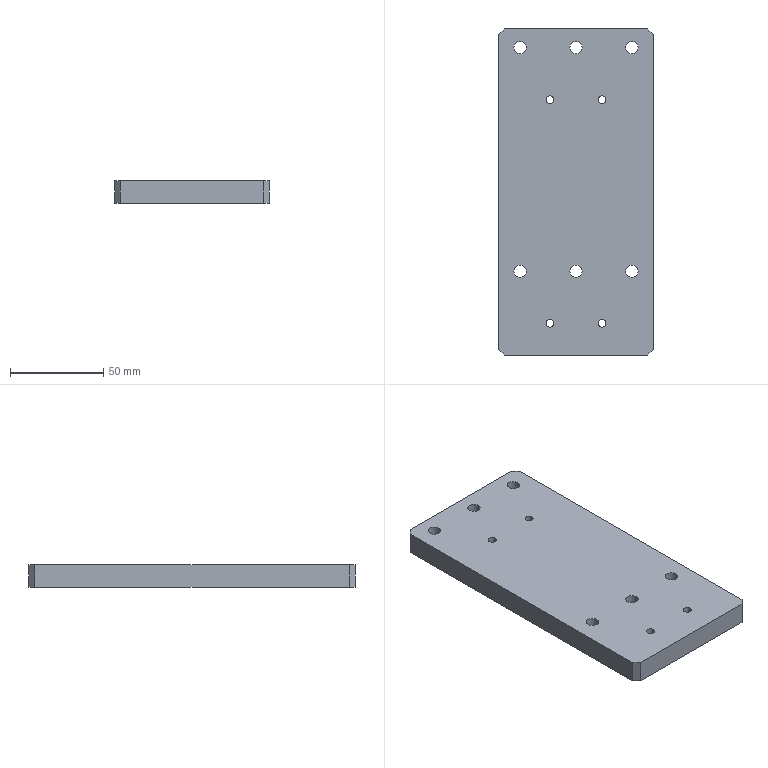Part | STEP file | 0-19-05 Lower cylinder mounting plate 2 | 1 solid | 48 faces | box 83 x 175 x 12 mm | volume 168474 mm3 | cylinder 32 | plane 16 | commonest cylinder face diameters 6.6 x12 11 x12 4.2 x8